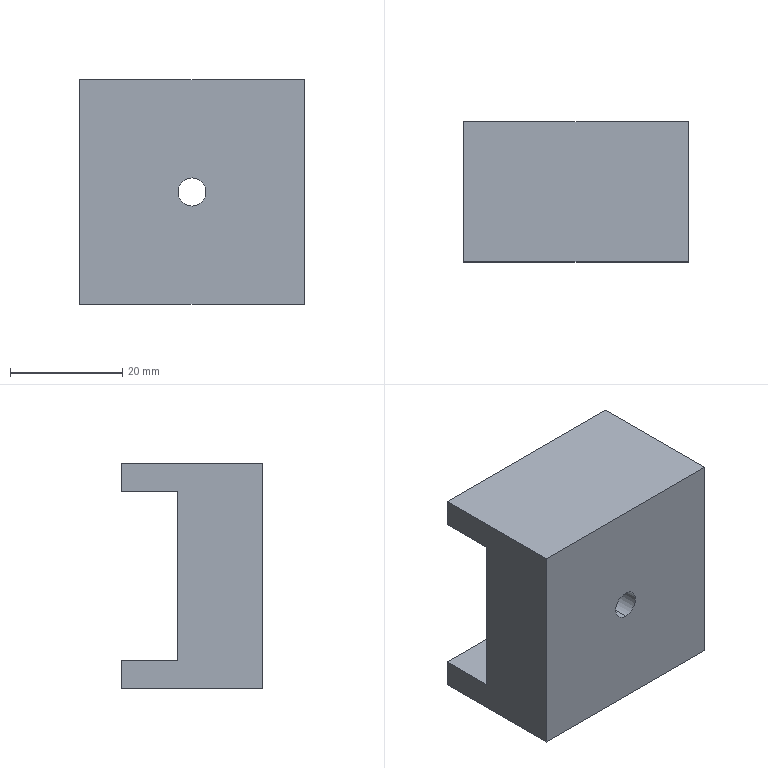Part | SolidWorks | features Extrusion 1, HoleWzd 1, ICE 1 | 1 solid | 12 faces | box 40 x 25 x 40 mm | volume 27705 mm3 | plane 10 | cylinder 2 | commonest cylinder face diameters 5 x2
STEP:
#1=CARTESIAN_POINT('',(0.,15.,2.5));
#2=VERTEX_POINT('',#1);
#3=CARTESIAN_POINT('',(0.,15.,-2.5));
#4=VERTEX_POINT('',#3);
#5=CARTESIAN_POINT('',(0.,15.,0.));
#6=DIRECTION('',(0.,-1.,0.));
#7=DIRECTION('',(0.,0.,-1.));
#8=AXIS2_PLACEMENT_3D('',#5,#6,#7);
#9=CIRCLE('',#8,2.5);
#10=EDGE_CURVE('',#2,#4,#9,.T.);
#11=ORIENTED_EDGE('',*,*,#10,.F.);
#12=CARTESIAN_POINT('',(0.,0.,2.5));
#13=VERTEX_POINT('',#12);
#14=CARTESIAN_POINT('',(0.,0.,2.5));
#15=DIRECTION('',(0.,-1.,0.));
#16=VECTOR('',#15,1000.);
#17=LINE('',#14,#16);
#18=EDGE_CURVE('',#2,#13,#17,.T.);
#19=ORIENTED_EDGE('',*,*,#18,.T.);
#20=CARTESIAN_POINT('',(0.,0.,-2.5));
#21=VERTEX_POINT('',#20);
#22=CARTESIAN_POINT('',(0.,0.,0.));
#23=DIRECTION('',(0.,-1.,0.));
#24=DIRECTION('',(0.,0.,-1.));
#25=AXIS2_PLACEMENT_3D('',#22,#23,#24);
#26=CIRCLE('',#25,2.5);
#27=EDGE_CURVE('',#13,#21,#26,.T.);
#28=ORIENTED_EDGE('',*,*,#27,.T.);
#29=CARTESIAN_POINT('',(0.,0.,-2.5));
#30=DIRECTION('',(0.,-1.,0.));
#31=VECTOR('',#30,1000.);
#32=LINE('',#29,#31);
#33=EDGE_CURVE('',#4,#21,#32,.T.);
#34=ORIENTED_EDGE('',*,*,#33,.F.);
#35=EDGE_LOOP('',(#11,#19,#28,#34));
#36=FACE_OUTER_BOUND('',#35,.T.);
#37=CARTESIAN_POINT('',(0.,0.,0.));
#38=DIRECTION('',(0.,-1.,0.));
#39=DIRECTION('',(0.,0.,-1.));
#40=AXIS2_PLACEMENT_3D('',#37,#38,#39);
#41=CYLINDRICAL_SURFACE('',#40,2.5);
#42=ADVANCED_FACE('',(#36),#41,.F.);
#43=CARTESIAN_POINT('',(-20.,25.,15.));
#44=VERTEX_POINT('',#43);
#45=CARTESIAN_POINT('',(20.,25.,15.));
#46=VERTEX_POINT('',#45);
#47=CARTESIAN_POINT('',(-20.,25.,15.));
#48=DIRECTION('',(1.,0.,0.));
#49=VECTOR('',#48,1000.);
#50=LINE('',#47,#49);
#51=EDGE_CURVE('',#44,#46,#50,.T.);
#52=ORIENTED_EDGE('',*,*,#51,.F.);
#53=CARTESIAN_POINT('',(-20.,25.,20.));
#54=VERTEX_POINT('',#53);
#55=CARTESIAN_POINT('',(-20.,25.,-20.));
#56=DIRECTION('',(0.,0.,1.));
#57=VECTOR('',#56,1000.);
#58=LINE('',#55,#57);
#59=EDGE_CURVE('',#44,#54,#58,.T.);
#60=ORIENTED_EDGE('',*,*,#59,.T.);
#61=CARTESIAN_POINT('',(20.,25.,20.));
#62=VERTEX_POINT('',#61);
#63=CARTESIAN_POINT('',(-20.,25.,20.));
#64=DIRECTION('',(1.,0.,0.));
#65=VECTOR('',#64,1000.);
#66=LINE('',#63,#65);
#67=EDGE_CURVE('',#54,#62,#66,.T.);
#68=ORIENTED_EDGE('',*,*,#67,.T.);
#69=CARTESIAN_POINT('',(20.,25.,-20.));
#70=DIRECTION('',(0.,0.,-1.));
#71=VECTOR('',#70,1000.);
#72=LINE('',#69,#71);
#73=EDGE_CURVE('',#62,#46,#72,.T.);
#74=ORIENTED_EDGE('',*,*,#73,.T.);
#75=EDGE_LOOP('',(#52,#60,#68,#74));
#76=FACE_OUTER_BOUND('',#75,.T.);
#77=CARTESIAN_POINT('',(0.,25.,0.));
#78=DIRECTION('',(0.,1.,0.));
#79=DIRECTION('',(0.,0.,1.));
#80=AXIS2_PLACEMENT_3D('',#77,#78,#79);
#81=PLANE('',#80);
#82=ADVANCED_FACE('',(#76),#81,.T.);
#83=CARTESIAN_POINT('',(20.,15.,15.));
#84=VERTEX_POINT('',#83);
#85=CARTESIAN_POINT('',(20.,15.,-15.));
#86=VERTEX_POINT('',#85);
#87=CARTESIAN_POINT('',(20.,15.,15.));
#88=DIRECTION('',(0.,0.,-1.));
#89=VECTOR('',#88,1000.);
#90=LINE('',#87,#89);
#91=EDGE_CURVE('',#84,#86,#90,.T.);
#92=ORIENTED_EDGE('',*,*,#91,.F.);
#93=CARTESIAN_POINT('',(20.,15.,15.));
#94=DIRECTION('',(0.,1.,0.));
#95=VECTOR('',#94,1000.);
#96=LINE('',#93,#95);
#97=EDGE_CURVE('',#84,#46,#96,.T.);
#98=ORIENTED_EDGE('',*,*,#97,.T.);
#99=ORIENTED_EDGE('',*,*,#73,.F.);
#100=CARTESIAN_POINT('',(20.,0.,20.));
#101=VERTEX_POINT('',#100);
#102=CARTESIAN_POINT('',(20.,25.,20.));
#103=DIRECTION('',(0.,-1.,0.));
#104=VECTOR('',#103,1000.);
#105=LINE('',#102,#104);
#106=EDGE_CURVE('',#62,#101,#105,.T.);
#107=ORIENTED_EDGE('',*,*,#106,.T.);
#108=CARTESIAN_POINT('',(20.,0.,-20.));
#109=VERTEX_POINT('',#108);
#110=CARTESIAN_POINT('',(20.,0.,-20.));
#111=DIRECTION('',(0.,0.,-1.));
#112=VECTOR('',#111,1000.);
#113=LINE('',#110,#112);
#114=EDGE_CURVE('',#101,#109,#113,.T.);
#115=ORIENTED_EDGE('',*,*,#114,.T.);
#116=CARTESIAN_POINT('',(20.,25.,-20.));
#117=VERTEX_POINT('',#116);
#118=CARTESIAN_POINT('',(20.,25.,-20.));
#119=DIRECTION('',(0.,-1.,0.));
#120=VECTOR('',#119,1000.);
#121=LINE('',#118,#120);
#122=EDGE_CURVE('',#117,#109,#121,.T.);
#123=ORIENTED_EDGE('',*,*,#122,.F.);
#124=CARTESIAN_POINT('',(20.,25.,-15.));
#125=VERTEX_POINT('',#124);
#126=CARTESIAN_POINT('',(20.,25.,-20.));
#127=DIRECTION('',(0.,0.,-1.));
#128=VECTOR('',#127,1000.);
#129=LINE('',#126,#128);
#130=EDGE_CURVE('',#125,#117,#129,.T.);
#131=ORIENTED_EDGE('',*,*,#130,.F.);
#132=CARTESIAN_POINT('',(20.,15.,-15.));
#133=DIRECTION('',(0.,1.,0.));
#134=VECTOR('',#133,1000.);
#135=LINE('',#132,#134);
#136=EDGE_CURVE('',#86,#125,#135,.T.);
#137=ORIENTED_EDGE('',*,*,#136,.F.);
#138=EDGE_LOOP('',(#92,#98,#99,#107,#115,#123,#131,#137));
#139=FACE_OUTER_BOUND('',#138,.T.);
#140=CARTESIAN_POINT('',(20.,25.,-20.));
#141=DIRECTION('',(-1.,0.,0.));
#142=DIRECTION('',(0.,0.,1.));
#143=AXIS2_PLACEMENT_3D('',#140,#141,#142);
#144=PLANE('',#143);
#145=ADVANCED_FACE('',(#139),#144,.F.);
#146=CARTESIAN_POINT('',(-20.,0.,-20.));
#147=VERTEX_POINT('',#146);
#148=CARTESIAN_POINT('',(-20.,0.,-20.));
#149=DIRECTION('',(-1.,0.,0.));
#150=VECTOR('',#149,1000.);
#151=LINE('',#148,#150);
#152=EDGE_CURVE('',#109,#147,#151,.T.);
#153=ORIENTED_EDGE('',*,*,#152,.T.);
#154=CARTESIAN_POINT('',(-20.,25.,-20.));
#155=VERTEX_POINT('',#154);
#156=CARTESIAN_POINT('',(-20.,25.,-20.));
#157=DIRECTION('',(0.,-1.,0.));
#158=VECTOR('',#157,1000.);
#159=LINE('',#156,#158);
#160=EDGE_CURVE('',#155,#147,#159,.T.);
#161=ORIENTED_EDGE('',*,*,#160,.F.);
#162=CARTESIAN_POINT('',(-20.,25.,-20.));
#163=DIRECTION('',(-1.,0.,0.));
#164=VECTOR('',#163,1000.);
#165=LINE('',#162,#164);
#166=EDGE_CURVE('',#117,#155,#165,.T.);
#167=ORIENTED_EDGE('',*,*,#166,.F.);
#168=ORIENTED_EDGE('',*,*,#122,.T.);
#169=EDGE_LOOP('',(#153,#161,#167,#168));
#170=FACE_OUTER_BOUND('',#169,.T.);
#171=CARTESIAN_POINT('',(-20.,25.,-20.));
#172=DIRECTION('',(0.,0.,1.));
#173=DIRECTION('',(1.,0.,0.));
#174=AXIS2_PLACEMENT_3D('',#171,#172,#173);
#175=PLANE('',#174);
#176=ADVANCED_FACE('',(#170),#175,.F.);
#177=ORIENTED_EDGE('',*,*,#59,.F.);
#178=CARTESIAN_POINT('',(-20.,15.,15.));
#179=VERTEX_POINT('',#178);
#180=CARTESIAN_POINT('',(-20.,15.,15.));
#181=DIRECTION('',(0.,1.,0.));
#182=VECTOR('',#181,1000.);
#183=LINE('',#180,#182);
#184=EDGE_CURVE('',#179,#44,#183,.T.);
#185=ORIENTED_EDGE('',*,*,#184,.F.);
#186=CARTESIAN_POINT('',(-20.,15.,-15.));
#187=VERTEX_POINT('',#186);
#188=CARTESIAN_POINT('',(-20.,15.,15.));
#189=DIRECTION('',(0.,0.,1.));
#190=VECTOR('',#189,1000.);
#191=LINE('',#188,#190);
#192=EDGE_CURVE('',#187,#179,#191,.T.);
#193=ORIENTED_EDGE('',*,*,#192,.F.);
#194=CARTESIAN_POINT('',(-20.,25.,-15.));
#195=VERTEX_POINT('',#194);
#196=CARTESIAN_POINT('',(-20.,15.,-15.));
#197=DIRECTION('',(0.,1.,0.));
#198=VECTOR('',#197,1000.);
#199=LINE('',#196,#198);
#200=EDGE_CURVE('',#187,#195,#199,.T.);
#201=ORIENTED_EDGE('',*,*,#200,.T.);
#202=CARTESIAN_POINT('',(-20.,25.,-20.));
#203=DIRECTION('',(0.,0.,1.));
#204=VECTOR('',#203,1000.);
#205=LINE('',#202,#204);
#206=EDGE_CURVE('',#155,#195,#205,.T.);
#207=ORIENTED_EDGE('',*,*,#206,.F.);
#208=ORIENTED_EDGE('',*,*,#160,.T.);
#209=CARTESIAN_POINT('',(-20.,0.,20.));
#210=VERTEX_POINT('',#209);
#211=CARTESIAN_POINT('',(-20.,0.,-20.));
#212=DIRECTION('',(0.,0.,1.));
#213=VECTOR('',#212,1000.);
#214=LINE('',#211,#213);
#215=EDGE_CURVE('',#147,#210,#214,.T.);
#216=ORIENTED_EDGE('',*,*,#215,.T.);
#217=CARTESIAN_POINT('',(-20.,25.,20.));
#218=DIRECTION('',(0.,-1.,0.));
#219=VECTOR('',#218,1000.);
#220=LINE('',#217,#219);
#221=EDGE_CURVE('',#54,#210,#220,.T.);
#222=ORIENTED_EDGE('',*,*,#221,.F.);
#223=EDGE_LOOP('',(#177,#185,#193,#201,#207,#208,#216,#222));
#224=FACE_OUTER_BOUND('',#223,.T.);
#225=CARTESIAN_POINT('',(-20.,25.,-20.));
#226=DIRECTION('',(1.,0.,0.));
#227=DIRECTION('',(0.,0.,-1.));
#228=AXIS2_PLACEMENT_3D('',#225,#226,#227);
#229=PLANE('',#228);
#230=ADVANCED_FACE('',(#224),#229,.F.);
#231=CARTESIAN_POINT('',(-20.,0.,20.));
#232=DIRECTION('',(1.,0.,0.));
#233=VECTOR('',#232,1000.);
#234=LINE('',#231,#233);
#235=EDGE_CURVE('',#210,#101,#234,.T.);
#236=ORIENTED_EDGE('',*,*,#235,.T.);
#237=ORIENTED_EDGE('',*,*,#106,.F.);
#238=ORIENTED_EDGE('',*,*,#67,.F.);
#239=ORIENTED_EDGE('',*,*,#221,.T.);
#240=EDGE_LOOP('',(#236,#237,#238,#239));
#241=FACE_OUTER_BOUND('',#240,.T.);
#242=CARTESIAN_POINT('',(-20.,25.,20.));
#243=DIRECTION('',(0.,0.,-1.));
#244=DIRECTION('',(-1.,0.,0.));
#245=AXIS2_PLACEMENT_3D('',#242,#243,#244);
#246=PLANE('',#245);
#247=ADVANCED_FACE('',(#241),#246,.F.);
#248=CARTESIAN_POINT('',(-20.,25.,-15.));
#249=DIRECTION('',(-1.,0.,0.));
#250=VECTOR('',#249,1000.);
#251=LINE('',#248,#250);
#252=EDGE_CURVE('',#125,#195,#251,.T.);
#253=ORIENTED_EDGE('',*,*,#252,.F.);
#254=ORIENTED_EDGE('',*,*,#130,.T.);
#255=ORIENTED_EDGE('',*,*,#166,.T.);
#256=ORIENTED_EDGE('',*,*,#206,.T.);
#257=EDGE_LOOP('',(#253,#254,#255,#256));
#258=FACE_OUTER_BOUND('',#257,.T.);
#259=CARTESIAN_POINT('',(0.,25.,0.));
#260=DIRECTION('',(0.,1.,0.));
#261=DIRECTION('',(0.,0.,1.));
#262=AXIS2_PLACEMENT_3D('',#259,#260,#261);
#263=PLANE('',#262);
#264=ADVANCED_FACE('',(#258),#263,.T.);
#265=CARTESIAN_POINT('',(0.,0.,0.));
#266=DIRECTION('',(0.,-1.,0.));
#267=DIRECTION('',(0.,0.,-1.));
#268=AXIS2_PLACEMENT_3D('',#265,#266,#267);
#269=CIRCLE('',#268,2.5);
#270=EDGE_CURVE('',#21,#13,#269,.T.);
#271=ORIENTED_EDGE('',*,*,#270,.F.);
#272=ORIENTED_EDGE('',*,*,#27,.F.);
#273=EDGE_LOOP('',(#271,#272));
#274=FACE_BOUND('',#273,.T.);
#275=ORIENTED_EDGE('',*,*,#114,.F.);
#276=ORIENTED_EDGE('',*,*,#235,.F.);
#277=ORIENTED_EDGE('',*,*,#215,.F.);
#278=ORIENTED_EDGE('',*,*,#152,.F.);
#279=EDGE_LOOP('',(#275,#276,#277,#278));
#280=FACE_OUTER_BOUND('',#279,.T.);
#281=CARTESIAN_POINT('',(0.,0.,0.));
#282=DIRECTION('',(0.,1.,0.));
#283=DIRECTION('',(0.,0.,1.));
#284=AXIS2_PLACEMENT_3D('',#281,#282,#283);
#285=PLANE('',#284);
#286=ADVANCED_FACE('',(#274,#280),#285,.F.);
#287=ORIENTED_EDGE('',*,*,#51,.T.);
#288=ORIENTED_EDGE('',*,*,#97,.F.);
#289=CARTESIAN_POINT('',(-20.,15.,15.));
#290=DIRECTION('',(1.,0.,0.));
#291=VECTOR('',#290,1000.);
#292=LINE('',#289,#291);
#293=EDGE_CURVE('',#179,#84,#292,.T.);
#294=ORIENTED_EDGE('',*,*,#293,.F.);
#295=ORIENTED_EDGE('',*,*,#184,.T.);
#296=EDGE_LOOP('',(#287,#288,#294,#295));
#297=FACE_OUTER_BOUND('',#296,.T.);
#298=CARTESIAN_POINT('',(-20.,15.,15.));
#299=DIRECTION('',(0.,0.,1.));
#300=DIRECTION('',(1.,0.,0.));
#301=AXIS2_PLACEMENT_3D('',#298,#299,#300);
#302=PLANE('',#301);
#303=ADVANCED_FACE('',(#297),#302,.F.);
#304=ORIENTED_EDGE('',*,*,#252,.T.);
#305=ORIENTED_EDGE('',*,*,#200,.F.);
#306=CARTESIAN_POINT('',(-20.,15.,-15.));
#307=DIRECTION('',(-1.,0.,0.));
#308=VECTOR('',#307,1000.);
#309=LINE('',#306,#308);
#310=EDGE_CURVE('',#86,#187,#309,.T.);
#311=ORIENTED_EDGE('',*,*,#310,.F.);
#312=ORIENTED_EDGE('',*,*,#136,.T.);
#313=EDGE_LOOP('',(#304,#305,#311,#312));
#314=FACE_OUTER_BOUND('',#313,.T.);
#315=CARTESIAN_POINT('',(-20.,15.,-15.));
#316=DIRECTION('',(0.,0.,-1.));
#317=DIRECTION('',(-1.,0.,0.));
#318=AXIS2_PLACEMENT_3D('',#315,#316,#317);
#319=PLANE('',#318);
#320=ADVANCED_FACE('',(#314),#319,.F.);
#321=CARTESIAN_POINT('',(0.,15.,0.));
#322=DIRECTION('',(0.,-1.,0.));
#323=DIRECTION('',(0.,0.,-1.));
#324=AXIS2_PLACEMENT_3D('',#321,#322,#323);
#325=CIRCLE('',#324,2.5);
#326=EDGE_CURVE('',#4,#2,#325,.T.);
#327=ORIENTED_EDGE('',*,*,#326,.T.);
#328=ORIENTED_EDGE('',*,*,#10,.T.);
#329=EDGE_LOOP('',(#327,#328));
#330=FACE_BOUND('',#329,.T.);
#331=ORIENTED_EDGE('',*,*,#91,.T.);
#332=ORIENTED_EDGE('',*,*,#310,.T.);
#333=ORIENTED_EDGE('',*,*,#192,.T.);
#334=ORIENTED_EDGE('',*,*,#293,.T.);
#335=EDGE_LOOP('',(#331,#332,#333,#334));
#336=FACE_OUTER_BOUND('',#335,.T.);
#337=CARTESIAN_POINT('',(0.,15.,0.));
#338=DIRECTION('',(0.,-1.,0.));
#339=DIRECTION('',(0.,0.,-1.));
#340=AXIS2_PLACEMENT_3D('',#337,#338,#339);
#341=PLANE('',#340);
#342=ADVANCED_FACE('',(#330,#336),#341,.F.);
#343=ORIENTED_EDGE('',*,*,#18,.F.);
#344=ORIENTED_EDGE('',*,*,#326,.F.);
#345=ORIENTED_EDGE('',*,*,#33,.T.);
#346=ORIENTED_EDGE('',*,*,#270,.T.);
#347=EDGE_LOOP('',(#343,#344,#345,#346));
#348=FACE_OUTER_BOUND('',#347,.T.);
#349=CARTESIAN_POINT('',(0.,0.,0.));
#350=DIRECTION('',(0.,-1.,0.));
#351=DIRECTION('',(0.,0.,-1.));
#352=AXIS2_PLACEMENT_3D('',#349,#350,#351);
#353=CYLINDRICAL_SURFACE('',#352,2.5);
#354=ADVANCED_FACE('',(#348),#353,.F.);
#355=CLOSED_SHELL('',(#42,#82,#145,#176,#230,#247,#264,#286,#303,#320,#342,#354));
#356=MANIFOLD_SOLID_BREP('',#355);
#357=CARTESIAN_POINT('',(0.,0.,0.));
#358=DIRECTION('',(0.,0.,1.));
#359=DIRECTION('',(1.,0.,0.));
#360=AXIS2_PLACEMENT_3D('',#357,#358,#359);
#361=(LENGTH_UNIT()NAMED_UNIT(*)SI_UNIT(.MILLI.,.METRE.));
#362=UNCERTAINTY_MEASURE_WITH_UNIT(LENGTH_MEASURE(0.00001),#361,'','');
#363=(NAMED_UNIT(*)PLANE_ANGLE_UNIT()SI_UNIT($,.RADIAN.));
#364=(NAMED_UNIT(*)SI_UNIT($,.STERADIAN.)SOLID_ANGLE_UNIT());
#365=(GEOMETRIC_REPRESENTATION_CONTEXT(3)GLOBAL_UNCERTAINTY_ASSIGNED_CONTEXT((#362))GLOBAL_UNIT_ASSIGNED_CONTEXT((#361,#363,#364))REPRESENTATION_CONTEXT('',''));
#366=ADVANCED_BREP_SHAPE_REPRESENTATION('',(#356,#360),#365);